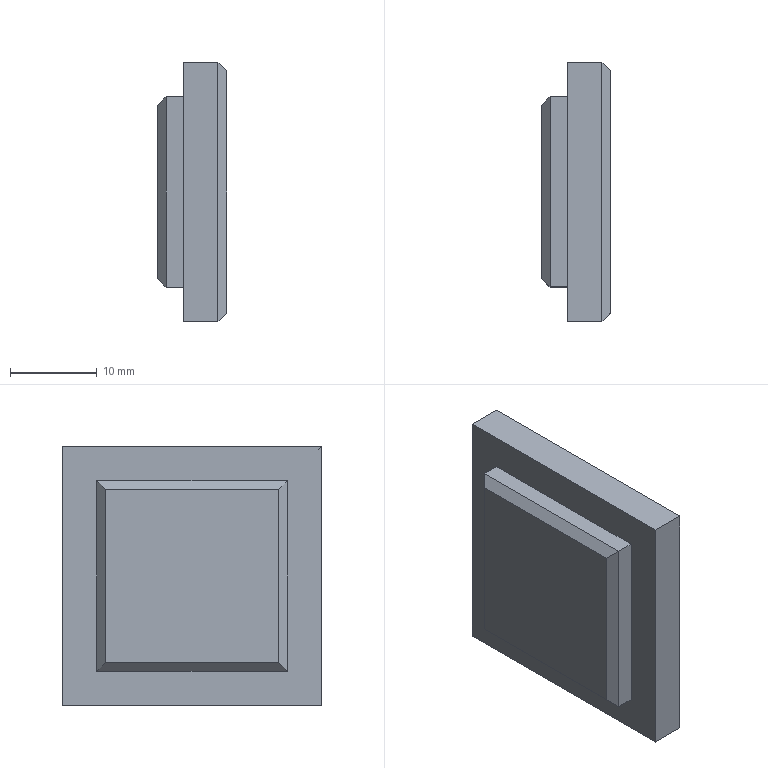Part | STEP file | profile cover | 1 solid | 19 faces | box 8 x 30 x 30 mm | volume 5851 mm3 | plane 19
STEP:
#1=CARTESIAN_POINT('',(120.,85.,15.));
#2=VERTEX_POINT('',#1);
#3=CARTESIAN_POINT('',(120.,55.,15.));
#4=VERTEX_POINT('',#3);
#5=CARTESIAN_POINT('',(120.,85.,15.));
#6=DIRECTION('',(0.,-1.,0.));
#7=VECTOR('',#6,1000.);
#8=LINE('',#5,#7);
#9=EDGE_CURVE('',#2,#4,#8,.T.);
#10=ORIENTED_EDGE('',*,*,#9,.F.);
#11=CARTESIAN_POINT('',(120.,85.,-15.));
#12=VERTEX_POINT('',#11);
#13=CARTESIAN_POINT('',(120.,85.,15.));
#14=DIRECTION('',(0.,0.,1.));
#15=VECTOR('',#14,1000.);
#16=LINE('',#13,#15);
#17=EDGE_CURVE('',#12,#2,#16,.T.);
#18=ORIENTED_EDGE('',*,*,#17,.F.);
#19=CARTESIAN_POINT('',(120.,55.,-15.));
#20=VERTEX_POINT('',#19);
#21=CARTESIAN_POINT('',(120.,85.,-15.));
#22=DIRECTION('',(0.,1.,0.));
#23=VECTOR('',#22,1000.);
#24=LINE('',#21,#23);
#25=EDGE_CURVE('',#20,#12,#24,.T.);
#26=ORIENTED_EDGE('',*,*,#25,.F.);
#27=CARTESIAN_POINT('',(120.,55.,15.));
#28=DIRECTION('',(0.,0.,-1.));
#29=VECTOR('',#28,1000.);
#30=LINE('',#27,#29);
#31=EDGE_CURVE('',#4,#20,#30,.T.);
#32=ORIENTED_EDGE('',*,*,#31,.F.);
#33=EDGE_LOOP('',(#10,#18,#26,#32));
#34=FACE_OUTER_BOUND('',#33,.T.);
#35=CARTESIAN_POINT('',(120.,59.,11.));
#36=VERTEX_POINT('',#35);
#37=CARTESIAN_POINT('',(120.,81.,11.));
#38=VERTEX_POINT('',#37);
#39=CARTESIAN_POINT('',(120.,59.,11.));
#40=DIRECTION('',(0.,1.,0.));
#41=VECTOR('',#40,1000.);
#42=LINE('',#39,#41);
#43=EDGE_CURVE('',#36,#38,#42,.T.);
#44=ORIENTED_EDGE('',*,*,#43,.F.);
#45=CARTESIAN_POINT('',(120.,59.,-11.));
#46=VERTEX_POINT('',#45);
#47=CARTESIAN_POINT('',(120.,59.,-11.));
#48=DIRECTION('',(0.,0.,1.));
#49=VECTOR('',#48,1000.);
#50=LINE('',#47,#49);
#51=EDGE_CURVE('',#46,#36,#50,.T.);
#52=ORIENTED_EDGE('',*,*,#51,.F.);
#53=CARTESIAN_POINT('',(120.,81.,-11.));
#54=VERTEX_POINT('',#53);
#55=CARTESIAN_POINT('',(120.,59.,-11.));
#56=DIRECTION('',(0.,-1.,0.));
#57=VECTOR('',#56,1000.);
#58=LINE('',#55,#57);
#59=EDGE_CURVE('',#54,#46,#58,.T.);
#60=ORIENTED_EDGE('',*,*,#59,.F.);
#61=CARTESIAN_POINT('',(120.,81.,-11.));
#62=DIRECTION('',(0.,0.,-1.));
#63=VECTOR('',#62,1000.);
#64=LINE('',#61,#63);
#65=EDGE_CURVE('',#38,#54,#64,.T.);
#66=ORIENTED_EDGE('',*,*,#65,.F.);
#67=EDGE_LOOP('',(#44,#52,#60,#66));
#68=FACE_BOUND('',#67,.T.);
#69=CARTESIAN_POINT('',(120.,55.,15.));
#70=DIRECTION('',(1.,0.,0.));
#71=DIRECTION('',(0.,0.,-1.));
#72=AXIS2_PLACEMENT_3D('',#69,#70,#71);
#73=PLANE('',#72);
#74=ADVANCED_FACE('',(#34,#68),#73,.F.);
#75=CARTESIAN_POINT('',(124.,55.,15.));
#76=VERTEX_POINT('',#75);
#77=CARTESIAN_POINT('',(125.,55.,15.));
#78=DIRECTION('',(-1.,0.,0.));
#79=VECTOR('',#78,1000.);
#80=LINE('',#77,#79);
#81=EDGE_CURVE('',#76,#4,#80,.T.);
#82=ORIENTED_EDGE('',*,*,#81,.F.);
#83=CARTESIAN_POINT('',(124.,85.,15.));
#84=VERTEX_POINT('',#83);
#85=CARTESIAN_POINT('',(124.,85.,15.));
#86=DIRECTION('',(0.,1.,0.));
#87=VECTOR('',#86,1000.);
#88=LINE('',#85,#87);
#89=EDGE_CURVE('',#76,#84,#88,.T.);
#90=ORIENTED_EDGE('',*,*,#89,.T.);
#91=CARTESIAN_POINT('',(125.,85.,15.));
#92=DIRECTION('',(-1.,0.,0.));
#93=VECTOR('',#92,1000.);
#94=LINE('',#91,#93);
#95=EDGE_CURVE('',#84,#2,#94,.T.);
#96=ORIENTED_EDGE('',*,*,#95,.T.);
#97=ORIENTED_EDGE('',*,*,#9,.T.);
#98=EDGE_LOOP('',(#82,#90,#96,#97));
#99=FACE_OUTER_BOUND('',#98,.T.);
#100=CARTESIAN_POINT('',(125.,85.,15.));
#101=DIRECTION('',(0.,0.,-1.));
#102=DIRECTION('',(0.,1.,0.));
#103=AXIS2_PLACEMENT_3D('',#100,#101,#102);
#104=PLANE('',#103);
#105=ADVANCED_FACE('',(#99),#104,.F.);
#106=CARTESIAN_POINT('',(124.,55.,-15.));
#107=VERTEX_POINT('',#106);
#108=CARTESIAN_POINT('',(125.,55.,-15.));
#109=DIRECTION('',(-1.,0.,0.));
#110=VECTOR('',#109,1000.);
#111=LINE('',#108,#110);
#112=EDGE_CURVE('',#107,#20,#111,.T.);
#113=ORIENTED_EDGE('',*,*,#112,.F.);
#114=CARTESIAN_POINT('',(124.,55.,15.));
#115=DIRECTION('',(0.,0.,1.));
#116=VECTOR('',#115,1000.);
#117=LINE('',#114,#116);
#118=EDGE_CURVE('',#107,#76,#117,.T.);
#119=ORIENTED_EDGE('',*,*,#118,.T.);
#120=ORIENTED_EDGE('',*,*,#81,.T.);
#121=ORIENTED_EDGE('',*,*,#31,.T.);
#122=EDGE_LOOP('',(#113,#119,#120,#121));
#123=FACE_OUTER_BOUND('',#122,.T.);
#124=CARTESIAN_POINT('',(125.,55.,15.));
#125=DIRECTION('',(0.,1.,0.));
#126=DIRECTION('',(0.,0.,1.));
#127=AXIS2_PLACEMENT_3D('',#124,#125,#126);
#128=PLANE('',#127);
#129=ADVANCED_FACE('',(#123),#128,.F.);
#130=CARTESIAN_POINT('',(124.,85.,-15.));
#131=VERTEX_POINT('',#130);
#132=CARTESIAN_POINT('',(125.,85.,-15.));
#133=DIRECTION('',(-1.,0.,0.));
#134=VECTOR('',#133,1000.);
#135=LINE('',#132,#134);
#136=EDGE_CURVE('',#131,#12,#135,.T.);
#137=ORIENTED_EDGE('',*,*,#136,.F.);
#138=CARTESIAN_POINT('',(124.,55.,-15.));
#139=DIRECTION('',(0.,-1.,0.));
#140=VECTOR('',#139,1000.);
#141=LINE('',#138,#140);
#142=EDGE_CURVE('',#131,#107,#141,.T.);
#143=ORIENTED_EDGE('',*,*,#142,.T.);
#144=ORIENTED_EDGE('',*,*,#112,.T.);
#145=ORIENTED_EDGE('',*,*,#25,.T.);
#146=EDGE_LOOP('',(#137,#143,#144,#145));
#147=FACE_OUTER_BOUND('',#146,.T.);
#148=CARTESIAN_POINT('',(125.,85.,-15.));
#149=DIRECTION('',(0.,0.,1.));
#150=DIRECTION('',(1.,0.,0.));
#151=AXIS2_PLACEMENT_3D('',#148,#149,#150);
#152=PLANE('',#151);
#153=ADVANCED_FACE('',(#147),#152,.F.);
#154=ORIENTED_EDGE('',*,*,#95,.F.);
#155=CARTESIAN_POINT('',(124.,85.,-15.));
#156=DIRECTION('',(0.,0.,-1.));
#157=VECTOR('',#156,1000.);
#158=LINE('',#155,#157);
#159=EDGE_CURVE('',#84,#131,#158,.T.);
#160=ORIENTED_EDGE('',*,*,#159,.T.);
#161=ORIENTED_EDGE('',*,*,#136,.T.);
#162=ORIENTED_EDGE('',*,*,#17,.T.);
#163=EDGE_LOOP('',(#154,#160,#161,#162));
#164=FACE_OUTER_BOUND('',#163,.T.);
#165=CARTESIAN_POINT('',(125.,85.,15.));
#166=DIRECTION('',(0.,-1.,0.));
#167=DIRECTION('',(0.,0.,-1.));
#168=AXIS2_PLACEMENT_3D('',#165,#166,#167);
#169=PLANE('',#168);
#170=ADVANCED_FACE('',(#164),#169,.F.);
#171=CARTESIAN_POINT('',(125.,84.,14.));
#172=VERTEX_POINT('',#171);
#173=CARTESIAN_POINT('',(125.,56.,14.));
#174=VERTEX_POINT('',#173);
#175=CARTESIAN_POINT('',(125.,55.,14.));
#176=DIRECTION('',(0.,-1.,0.));
#177=VECTOR('',#176,1000.);
#178=LINE('',#175,#177);
#179=EDGE_CURVE('',#172,#174,#178,.T.);
#180=ORIENTED_EDGE('',*,*,#179,.T.);
#181=CARTESIAN_POINT('',(125.,56.,-14.));
#182=VERTEX_POINT('',#181);
#183=CARTESIAN_POINT('',(125.,56.,-15.));
#184=DIRECTION('',(0.,0.,-1.));
#185=VECTOR('',#184,1000.);
#186=LINE('',#183,#185);
#187=EDGE_CURVE('',#174,#182,#186,.T.);
#188=ORIENTED_EDGE('',*,*,#187,.T.);
#189=CARTESIAN_POINT('',(125.,84.,-14.));
#190=VERTEX_POINT('',#189);
#191=CARTESIAN_POINT('',(125.,85.,-14.));
#192=DIRECTION('',(0.,1.,0.));
#193=VECTOR('',#192,1000.);
#194=LINE('',#191,#193);
#195=EDGE_CURVE('',#182,#190,#194,.T.);
#196=ORIENTED_EDGE('',*,*,#195,.T.);
#197=CARTESIAN_POINT('',(125.,84.,15.));
#198=DIRECTION('',(0.,0.,1.));
#199=VECTOR('',#198,1000.);
#200=LINE('',#197,#199);
#201=EDGE_CURVE('',#190,#172,#200,.T.);
#202=ORIENTED_EDGE('',*,*,#201,.T.);
#203=EDGE_LOOP('',(#180,#188,#196,#202));
#204=FACE_OUTER_BOUND('',#203,.T.);
#205=CARTESIAN_POINT('',(125.,55.,15.));
#206=DIRECTION('',(1.,0.,0.));
#207=DIRECTION('',(0.,0.,-1.));
#208=AXIS2_PLACEMENT_3D('',#205,#206,#207);
#209=PLANE('',#208);
#210=ADVANCED_FACE('',(#204),#209,.T.);
#211=CARTESIAN_POINT('',(118.,81.,11.));
#212=VERTEX_POINT('',#211);
#213=CARTESIAN_POINT('',(117.,81.,11.));
#214=DIRECTION('',(1.,0.,0.));
#215=VECTOR('',#214,1000.);
#216=LINE('',#213,#215);
#217=EDGE_CURVE('',#212,#38,#216,.T.);
#218=ORIENTED_EDGE('',*,*,#217,.F.);
#219=CARTESIAN_POINT('',(118.,59.,11.));
#220=VERTEX_POINT('',#219);
#221=CARTESIAN_POINT('',(118.,59.,11.));
#222=DIRECTION('',(0.,-1.,0.));
#223=VECTOR('',#222,1000.);
#224=LINE('',#221,#223);
#225=EDGE_CURVE('',#212,#220,#224,.T.);
#226=ORIENTED_EDGE('',*,*,#225,.T.);
#227=CARTESIAN_POINT('',(117.,59.,11.));
#228=DIRECTION('',(1.,0.,0.));
#229=VECTOR('',#228,1000.);
#230=LINE('',#227,#229);
#231=EDGE_CURVE('',#220,#36,#230,.T.);
#232=ORIENTED_EDGE('',*,*,#231,.T.);
#233=ORIENTED_EDGE('',*,*,#43,.T.);
#234=EDGE_LOOP('',(#218,#226,#232,#233));
#235=FACE_OUTER_BOUND('',#234,.T.);
#236=CARTESIAN_POINT('',(117.,59.,11.));
#237=DIRECTION('',(0.,0.,-1.));
#238=DIRECTION('',(-1.,0.,0.));
#239=AXIS2_PLACEMENT_3D('',#236,#237,#238);
#240=PLANE('',#239);
#241=ADVANCED_FACE('',(#235),#240,.F.);
#242=CARTESIAN_POINT('',(118.,81.,-11.));
#243=VERTEX_POINT('',#242);
#244=CARTESIAN_POINT('',(117.,81.,-11.));
#245=DIRECTION('',(1.,0.,0.));
#246=VECTOR('',#245,1000.);
#247=LINE('',#244,#246);
#248=EDGE_CURVE('',#243,#54,#247,.T.);
#249=ORIENTED_EDGE('',*,*,#248,.F.);
#250=CARTESIAN_POINT('',(118.,81.,-11.));
#251=DIRECTION('',(0.,0.,1.));
#252=VECTOR('',#251,1000.);
#253=LINE('',#250,#252);
#254=EDGE_CURVE('',#243,#212,#253,.T.);
#255=ORIENTED_EDGE('',*,*,#254,.T.);
#256=ORIENTED_EDGE('',*,*,#217,.T.);
#257=ORIENTED_EDGE('',*,*,#65,.T.);
#258=EDGE_LOOP('',(#249,#255,#256,#257));
#259=FACE_OUTER_BOUND('',#258,.T.);
#260=CARTESIAN_POINT('',(117.,81.,-11.));
#261=DIRECTION('',(0.,-1.,0.));
#262=DIRECTION('',(0.,0.,-1.));
#263=AXIS2_PLACEMENT_3D('',#260,#261,#262);
#264=PLANE('',#263);
#265=ADVANCED_FACE('',(#259),#264,.F.);
#266=CARTESIAN_POINT('',(118.,59.,-11.));
#267=VERTEX_POINT('',#266);
#268=CARTESIAN_POINT('',(117.,59.,-11.));
#269=DIRECTION('',(1.,0.,0.));
#270=VECTOR('',#269,1000.);
#271=LINE('',#268,#270);
#272=EDGE_CURVE('',#267,#46,#271,.T.);
#273=ORIENTED_EDGE('',*,*,#272,.F.);
#274=CARTESIAN_POINT('',(118.,59.,-11.));
#275=DIRECTION('',(0.,1.,0.));
#276=VECTOR('',#275,1000.);
#277=LINE('',#274,#276);
#278=EDGE_CURVE('',#267,#243,#277,.T.);
#279=ORIENTED_EDGE('',*,*,#278,.T.);
#280=ORIENTED_EDGE('',*,*,#248,.T.);
#281=ORIENTED_EDGE('',*,*,#59,.T.);
#282=EDGE_LOOP('',(#273,#279,#280,#281));
#283=FACE_OUTER_BOUND('',#282,.T.);
#284=CARTESIAN_POINT('',(117.,59.,-11.));
#285=DIRECTION('',(0.,0.,1.));
#286=DIRECTION('',(1.,0.,0.));
#287=AXIS2_PLACEMENT_3D('',#284,#285,#286);
#288=PLANE('',#287);
#289=ADVANCED_FACE('',(#283),#288,.F.);
#290=ORIENTED_EDGE('',*,*,#231,.F.);
#291=CARTESIAN_POINT('',(118.,59.,-11.));
#292=DIRECTION('',(0.,0.,-1.));
#293=VECTOR('',#292,1000.);
#294=LINE('',#291,#293);
#295=EDGE_CURVE('',#220,#267,#294,.T.);
#296=ORIENTED_EDGE('',*,*,#295,.T.);
#297=ORIENTED_EDGE('',*,*,#272,.T.);
#298=ORIENTED_EDGE('',*,*,#51,.T.);
#299=EDGE_LOOP('',(#290,#296,#297,#298));
#300=FACE_OUTER_BOUND('',#299,.T.);
#301=CARTESIAN_POINT('',(117.,59.,-11.));
#302=DIRECTION('',(0.,1.,0.));
#303=DIRECTION('',(0.,0.,1.));
#304=AXIS2_PLACEMENT_3D('',#301,#302,#303);
#305=PLANE('',#304);
#306=ADVANCED_FACE('',(#300),#305,.F.);
#307=CARTESIAN_POINT('',(117.,80.,-10.));
#308=VERTEX_POINT('',#307);
#309=CARTESIAN_POINT('',(117.,60.,-10.));
#310=VERTEX_POINT('',#309);
#311=CARTESIAN_POINT('',(117.,81.,-10.));
#312=DIRECTION('',(0.,-1.,0.));
#313=VECTOR('',#312,1000.);
#314=LINE('',#311,#313);
#315=EDGE_CURVE('',#308,#310,#314,.T.);
#316=ORIENTED_EDGE('',*,*,#315,.T.);
#317=CARTESIAN_POINT('',(117.,60.,10.));
#318=VERTEX_POINT('',#317);
#319=CARTESIAN_POINT('',(117.,60.,11.));
#320=DIRECTION('',(0.,0.,1.));
#321=VECTOR('',#320,1000.);
#322=LINE('',#319,#321);
#323=EDGE_CURVE('',#310,#318,#322,.T.);
#324=ORIENTED_EDGE('',*,*,#323,.T.);
#325=CARTESIAN_POINT('',(117.,80.,10.));
#326=VERTEX_POINT('',#325);
#327=CARTESIAN_POINT('',(117.,81.,10.));
#328=DIRECTION('',(0.,1.,0.));
#329=VECTOR('',#328,1000.);
#330=LINE('',#327,#329);
#331=EDGE_CURVE('',#318,#326,#330,.T.);
#332=ORIENTED_EDGE('',*,*,#331,.T.);
#333=CARTESIAN_POINT('',(117.,80.,11.));
#334=DIRECTION('',(0.,0.,-1.));
#335=VECTOR('',#334,1000.);
#336=LINE('',#333,#335);
#337=EDGE_CURVE('',#326,#308,#336,.T.);
#338=ORIENTED_EDGE('',*,*,#337,.T.);
#339=EDGE_LOOP('',(#316,#324,#332,#338));
#340=FACE_OUTER_BOUND('',#339,.T.);
#341=CARTESIAN_POINT('',(117.,81.,11.));
#342=DIRECTION('',(1.,0.,0.));
#343=DIRECTION('',(0.,0.,-1.));
#344=AXIS2_PLACEMENT_3D('',#341,#342,#343);
#345=PLANE('',#344);
#346=ADVANCED_FACE('',(#340),#345,.F.);
#347=CARTESIAN_POINT('',(117.333,80.333,10.333));
#348=DIRECTION('',(-0.5774,-0.5774,-0.5774));
#349=VECTOR('',#348,1000.);
#350=LINE('',#347,#349);
#351=EDGE_CURVE('',#212,#326,#350,.T.);
#352=ORIENTED_EDGE('',*,*,#351,.F.);
#353=ORIENTED_EDGE('',*,*,#254,.F.);
#354=CARTESIAN_POINT('',(110.,73.,-3.));
#355=DIRECTION('',(0.5774,0.5774,-0.5774));
#356=VECTOR('',#355,1000.);
#357=LINE('',#354,#356);
#358=EDGE_CURVE('',#308,#243,#357,.T.);
#359=ORIENTED_EDGE('',*,*,#358,.F.);
#360=ORIENTED_EDGE('',*,*,#337,.F.);
#361=EDGE_LOOP('',(#352,#353,#359,#360));
#362=FACE_OUTER_BOUND('',#361,.T.);
#363=CARTESIAN_POINT('',(117.,80.,11.));
#364=DIRECTION('',(0.7071,-0.7071,0.));
#365=DIRECTION('',(0.7071,0.7071,0.));
#366=AXIS2_PLACEMENT_3D('',#363,#364,#365);
#367=PLANE('',#366);
#368=ADVANCED_FACE('',(#362),#367,.F.);
#369=ORIENTED_EDGE('',*,*,#358,.T.);
#370=ORIENTED_EDGE('',*,*,#278,.F.);
#371=CARTESIAN_POINT('',(110.,67.,-3.));
#372=DIRECTION('',(0.5774,-0.5774,-0.5774));
#373=VECTOR('',#372,1000.);
#374=LINE('',#371,#373);
#375=EDGE_CURVE('',#310,#267,#374,.T.);
#376=ORIENTED_EDGE('',*,*,#375,.F.);
#377=ORIENTED_EDGE('',*,*,#315,.F.);
#378=EDGE_LOOP('',(#369,#370,#376,#377));
#379=FACE_OUTER_BOUND('',#378,.T.);
#380=CARTESIAN_POINT('',(117.,81.,-10.));
#381=DIRECTION('',(0.7071,0.,0.7071));
#382=DIRECTION('',(0.7071,0.,-0.7071));
#383=AXIS2_PLACEMENT_3D('',#380,#381,#382);
#384=PLANE('',#383);
#385=ADVANCED_FACE('',(#379),#384,.F.);
#386=ORIENTED_EDGE('',*,*,#351,.T.);
#387=ORIENTED_EDGE('',*,*,#331,.F.);
#388=CARTESIAN_POINT('',(110.,67.,3.));
#389=DIRECTION('',(-0.5774,0.5774,-0.5774));
#390=VECTOR('',#389,1000.);
#391=LINE('',#388,#390);
#392=EDGE_CURVE('',#220,#318,#391,.T.);
#393=ORIENTED_EDGE('',*,*,#392,.F.);
#394=ORIENTED_EDGE('',*,*,#225,.F.);
#395=EDGE_LOOP('',(#386,#387,#393,#394));
#396=FACE_OUTER_BOUND('',#395,.T.);
#397=CARTESIAN_POINT('',(117.,81.,10.));
#398=DIRECTION('',(0.7071,0.,-0.7071));
#399=DIRECTION('',(-0.7071,0.,-0.7071));
#400=AXIS2_PLACEMENT_3D('',#397,#398,#399);
#401=PLANE('',#400);
#402=ADVANCED_FACE('',(#396),#401,.F.);
#403=ORIENTED_EDGE('',*,*,#375,.T.);
#404=ORIENTED_EDGE('',*,*,#295,.F.);
#405=ORIENTED_EDGE('',*,*,#392,.T.);
#406=ORIENTED_EDGE('',*,*,#323,.F.);
#407=EDGE_LOOP('',(#403,#404,#405,#406));
#408=FACE_OUTER_BOUND('',#407,.T.);
#409=CARTESIAN_POINT('',(117.,60.,11.));
#410=DIRECTION('',(0.7071,0.7071,0.));
#411=DIRECTION('',(-0.7071,0.7071,0.));
#412=AXIS2_PLACEMENT_3D('',#409,#410,#411);
#413=PLANE('',#412);
#414=ADVANCED_FACE('',(#408),#413,.F.);
#415=CARTESIAN_POINT('',(134.667,74.333,-4.333));
#416=DIRECTION('',(0.5774,-0.5774,0.5774));
#417=VECTOR('',#416,1000.);
#418=LINE('',#415,#417);
#419=EDGE_CURVE('',#131,#190,#418,.T.);
#420=ORIENTED_EDGE('',*,*,#419,.F.);
#421=ORIENTED_EDGE('',*,*,#159,.F.);
#422=CARTESIAN_POINT('',(124.667,84.333,14.333));
#423=DIRECTION('',(-0.5774,0.5774,0.5774));
#424=VECTOR('',#423,1000.);
#425=LINE('',#422,#424);
#426=EDGE_CURVE('',#172,#84,#425,.T.);
#427=ORIENTED_EDGE('',*,*,#426,.F.);
#428=ORIENTED_EDGE('',*,*,#201,.F.);
#429=EDGE_LOOP('',(#420,#421,#427,#428));
#430=FACE_OUTER_BOUND('',#429,.T.);
#431=CARTESIAN_POINT('',(125.,84.,15.));
#432=DIRECTION('',(0.7071,0.7071,0.));
#433=DIRECTION('',(-0.7071,0.7071,0.));
#434=AXIS2_PLACEMENT_3D('',#431,#432,#433);
#435=PLANE('',#434);
#436=ADVANCED_FACE('',(#430),#435,.T.);
#437=ORIENTED_EDGE('',*,*,#426,.T.);
#438=ORIENTED_EDGE('',*,*,#89,.F.);
#439=CARTESIAN_POINT('',(124.667,55.667,14.333));
#440=DIRECTION('',(-0.5774,-0.5774,0.5774));
#441=VECTOR('',#440,1000.);
#442=LINE('',#439,#441);
#443=EDGE_CURVE('',#174,#76,#442,.T.);
#444=ORIENTED_EDGE('',*,*,#443,.F.);
#445=ORIENTED_EDGE('',*,*,#179,.F.);
#446=EDGE_LOOP('',(#437,#438,#444,#445));
#447=FACE_OUTER_BOUND('',#446,.T.);
#448=CARTESIAN_POINT('',(125.,55.,14.));
#449=DIRECTION('',(0.7071,0.,0.7071));
#450=DIRECTION('',(0.7071,0.,-0.7071));
#451=AXIS2_PLACEMENT_3D('',#448,#449,#450);
#452=PLANE('',#451);
#453=ADVANCED_FACE('',(#447),#452,.T.);
#454=ORIENTED_EDGE('',*,*,#419,.T.);
#455=ORIENTED_EDGE('',*,*,#195,.F.);
#456=CARTESIAN_POINT('',(124.667,55.667,-14.333));
#457=DIRECTION('',(0.5774,0.5774,0.5774));
#458=VECTOR('',#457,1000.);
#459=LINE('',#456,#458);
#460=EDGE_CURVE('',#107,#182,#459,.T.);
#461=ORIENTED_EDGE('',*,*,#460,.F.);
#462=ORIENTED_EDGE('',*,*,#142,.F.);
#463=EDGE_LOOP('',(#454,#455,#461,#462));
#464=FACE_OUTER_BOUND('',#463,.T.);
#465=CARTESIAN_POINT('',(125.,55.,-14.));
#466=DIRECTION('',(0.7071,0.,-0.7071));
#467=DIRECTION('',(-0.7071,0.,-0.7071));
#468=AXIS2_PLACEMENT_3D('',#465,#466,#467);
#469=PLANE('',#468);
#470=ADVANCED_FACE('',(#464),#469,.T.);
#471=ORIENTED_EDGE('',*,*,#443,.T.);
#472=ORIENTED_EDGE('',*,*,#118,.F.);
#473=ORIENTED_EDGE('',*,*,#460,.T.);
#474=ORIENTED_EDGE('',*,*,#187,.F.);
#475=EDGE_LOOP('',(#471,#472,#473,#474));
#476=FACE_OUTER_BOUND('',#475,.T.);
#477=CARTESIAN_POINT('',(125.,56.,15.));
#478=DIRECTION('',(0.7071,-0.7071,0.));
#479=DIRECTION('',(0.7071,0.7071,0.));
#480=AXIS2_PLACEMENT_3D('',#477,#478,#479);
#481=PLANE('',#480);
#482=ADVANCED_FACE('',(#476),#481,.T.);
#483=CLOSED_SHELL('',(#74,#105,#129,#153,#170,#210,#241,#265,#289,#306,#346,#368,#385,#402,#414,#436,#453,#470,#482));
#484=MANIFOLD_SOLID_BREP('',#483);
#485=CARTESIAN_POINT('',(0.,0.,0.));
#486=DIRECTION('',(0.,0.,1.));
#487=DIRECTION('',(1.,0.,0.));
#488=AXIS2_PLACEMENT_3D('',#485,#486,#487);
#489=(LENGTH_UNIT()NAMED_UNIT(*)SI_UNIT(.MILLI.,.METRE.));
#490=UNCERTAINTY_MEASURE_WITH_UNIT(LENGTH_MEASURE(0.00001),#489,'','');
#491=(NAMED_UNIT(*)PLANE_ANGLE_UNIT()SI_UNIT($,.RADIAN.));
#492=(NAMED_UNIT(*)SI_UNIT($,.STERADIAN.)SOLID_ANGLE_UNIT());
#493=(GEOMETRIC_REPRESENTATION_CONTEXT(3)GLOBAL_UNCERTAINTY_ASSIGNED_CONTEXT((#490))GLOBAL_UNIT_ASSIGNED_CONTEXT((#489,#491,#492))REPRESENTATION_CONTEXT('',''));
#494=ADVANCED_BREP_SHAPE_REPRESENTATION('',(#484,#488),#493);